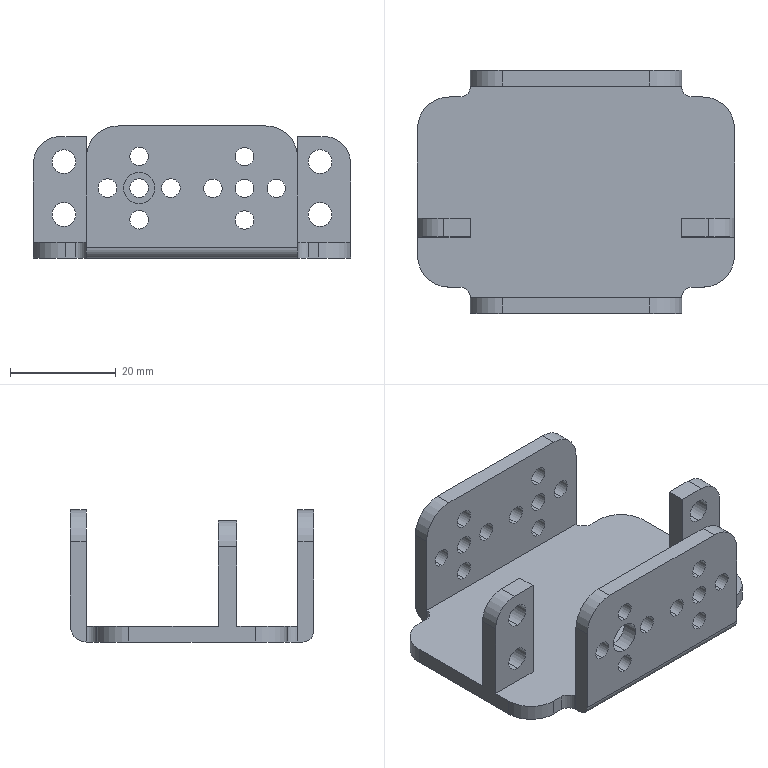Part | SolidWorks | features Fillet 7, Cut 5, ICE 2, Extrusion 1, MirrorPattern 1 | 1 solid | 90 faces | box 60 x 46 x 25 mm | volume 13187 mm3 | cylinder 64 | plane 26 | commonest cylinder face diameters 3.5 x38 4.5 x8 12 x8 4 x5 5.94 x2 10 x2